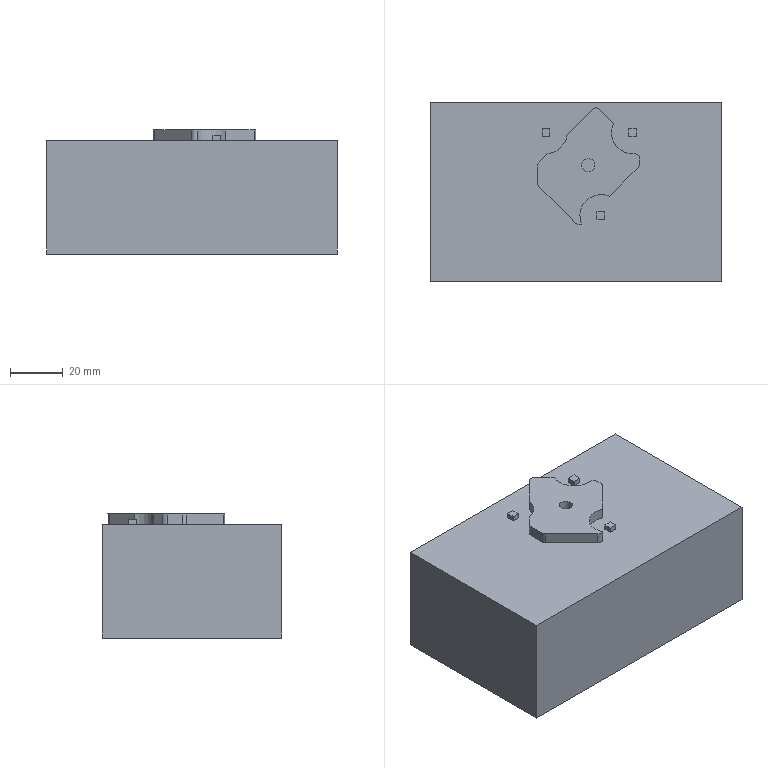NC program | NX | posted with a generic post | part box 110.151 x 68.163 x 47.1 mm
Lines 3425 to 4268 of 32691:
(PLANAR_MILL_2 , TOOL : D4R0)
N6680 T14 M6
N6682 G54
N6684 G17 G0 G90 X46.442 Y26.396 S5000 M3
N6686 G43 Z80. H14
N6688 G94 G1 Z0.5 F5000.
N6690 X46.014 Y26.643 Z0.487 F1500.
N6692 X45.498 Y26.638 Z0.474
N6694 X45.082 Y26.398 Z0.461
N6696 X44.819 Y25.953 Z0.447
N6698 Y25.437 Z0.434
N6700 X45.082 Y24.993 Z0.42
N6702 X45.498 Y24.752 Z0.408
N6704 X46.014 Y24.748 Z0.394
N6706 X46.461 Y25.005 Z0.381
N6708 X46.715 Y25.455 Z0.367
N6710 Y25.936 Z0.355
N6712 X46.461 Y26.385 Z0.341
N6714 X46.014 Y26.643 Z0.328
N6716 X45.498 Y26.638 Z0.314
N6718 X45.082 Y26.398 Z0.302
N6720 X44.819 Y25.953 Z0.288
N6722 Y25.437 Z0.275
N6724 X45.082 Y24.993 Z0.261
N6726 X45.498 Y24.752 Z0.248
N6728 X46.014 Y24.748 Z0.235
N6730 X46.461 Y25.005 Z0.221
N6732 X46.715 Y25.455 Z0.208
N6734 Y25.936 Z0.195
N6736 X46.461 Y26.385 Z0.182
N6738 X46.014 Y26.643 Z0.168
N6740 X45.498 Y26.638 Z0.155
N6742 X45.082 Y26.398 Z0.142
N6744 X44.819 Y25.953 Z0.129
N6746 Y25.437 Z0.115
N6748 X45.082 Y24.993 Z0.102
N6750 X45.498 Y24.752 Z0.089
N6752 X46.014 Y24.748 Z0.076
N6754 X46.461 Y25.005 Z0.062
N6756 X46.715 Y25.455 Z0.048
N6758 Y25.936 Z0.036
N6760 X46.461 Y26.385 Z0.022
N6762 X46.014 Y26.643 Z0.009
N6764 X45.498 Y26.638 Z-0.005
N6766 X45.082 Y26.398 Z-0.017
N6768 X44.819 Y25.953 Z-0.031
N6770 Y25.437 Z-0.044
N6772 X45.082 Y24.993 Z-0.058
N6774 X45.498 Y24.752 Z-0.07
N6776 X46.014 Y24.748 Z-0.084
N6778 X46.461 Y25.005 Z-0.097
N6780 X46.715 Y25.455 Z-0.111
N6782 Y25.936 Z-0.124
N6784 X46.461 Y26.385 Z-0.137
N6786 X46.014 Y26.643 Z-0.151
N6788 X45.498 Y26.638 Z-0.164
N6790 X45.082 Y26.398 Z-0.177
N6792 X44.819 Y25.953 Z-0.19
N6794 Y25.437 Z-0.204
N6796 X45.082 Y24.993 Z-0.217
N6798 X45.498 Y24.752 Z-0.23
N6800 X46.014 Y24.748 Z-0.243
N6802 X46.461 Y25.005 Z-0.257
N6804 X46.715 Y25.455 Z-0.27
N6806 Y25.936 Z-0.283
N6808 X46.461 Y26.385 Z-0.296
N6810 X46.014 Y26.643 Z-0.31
N6812 X45.498 Y26.638 Z-0.323
N6814 X45.082 Y26.398 Z-0.336
N6816 X44.819 Y25.953 Z-0.35
N6818 Y25.437 Z-0.363
N6820 X45.082 Y24.993 Z-0.377
N6822 X45.498 Y24.752 Z-0.389
N6824 X46.014 Y24.748 Z-0.403
N6826 X46.461 Y25.005 Z-0.416
N6828 X46.715 Y25.455 Z-0.43
N6830 Y25.936 Z-0.442
N6832 X46.461 Y26.385 Z-0.456
N6834 X46.014 Y26.643 Z-0.469
N6836 X45.498 Y26.638 Z-0.483
N6838 X45.082 Y26.398 Z-0.495
N6840 X44.819 Y25.953 Z-0.509
N6842 Y25.437 Z-0.522
N6844 X45.082 Y24.993 Z-0.536
N6846 X45.498 Y24.752 Z-0.549
N6848 X46.014 Y24.748 Z-0.562
N6850 X46.461 Y25.005 Z-0.576
N6852 X46.715 Y25.455 Z-0.589
N6854 Y25.936 Z-0.602
N6856 X46.461 Y26.385 Z-0.615
N6858 X46.014 Y26.643 Z-0.629
N6860 X45.498 Y26.638 Z-0.642
N6862 X45.082 Y26.398 Z-0.655
N6864 X44.819 Y25.953 Z-0.668
N6866 Y25.437 Z-0.682
N6868 X45.082 Y24.993 Z-0.695
N6870 X45.498 Y24.752 Z-0.708
N6872 X46.014 Y24.748 Z-0.721
N6874 X46.461 Y25.005 Z-0.735
N6876 X46.715 Y25.455 Z-0.749
N6878 Y25.936 Z-0.761
N6880 X46.461 Y26.385 Z-0.775
N6882 X46.014 Y26.643 Z-0.788
N6884 X45.498 Y26.638 Z-0.802
N6886 X45.082 Y26.398 Z-0.814
N6888 X44.819 Y25.953 Z-0.828
N6890 Y25.437 Z-0.841
N6892 X45.082 Y24.993 Z-0.855
N6894 X45.498 Y24.752 Z-0.867
N6896 X46.014 Y24.748 Z-0.881
N6898 X46.461 Y25.005 Z-0.894
N6900 X46.715 Y25.455 Z-0.908
N6902 Y25.936 Z-0.921
N6904 X46.461 Y26.385 Z-0.934
N6906 X46.014 Y26.643 Z-0.948
N6908 X45.498 Y26.638 Z-0.961
N6910 X45.082 Y26.398 Z-0.974
N6912 X44.819 Y25.953 Z-0.987
N6914 Y25.437 Z-1.001
N6916 X45.082 Y24.993 Z-1.014
N6918 X45.498 Y24.752 Z-1.027
N6920 X46.014 Y24.748 Z-1.04
N6922 X46.461 Y25.005 Z-1.054
N6924 X46.715 Y25.455 Z-1.067
N6926 Y25.936 Z-1.08
N6928 X46.461 Y26.385 Z-1.093
N6930 X46.014 Y26.643 Z-1.107
N6932 X45.498 Y26.638 Z-1.12
N6934 X45.082 Y26.398 Z-1.133
N6936 X44.819 Y25.953 Z-1.147
N6938 Y25.437 Z-1.16
N6940 X45.082 Y24.993 Z-1.174
N6942 X45.498 Y24.752 Z-1.186
N6944 X46.014 Y24.748 Z-1.2
N6946 X46.461 Y25.005 Z-1.213
N6948 X46.715 Y25.455 Z-1.227
N6950 Y25.936 Z-1.239
N6952 X46.461 Y26.385 Z-1.253
N6954 X46.014 Y26.643 Z-1.266
N6956 X45.498 Y26.638 Z-1.28
N6958 X45.082 Y26.398 Z-1.292
N6960 X44.819 Y25.953 Z-1.306
N6962 Y25.437 Z-1.319
N6964 X45.082 Y24.993 Z-1.333
N6966 X45.498 Y24.752 Z-1.346
N6968 X46.014 Y24.748 Z-1.359
N6970 X46.461 Y25.005 Z-1.373
N6972 X46.715 Y25.455 Z-1.386
N6974 Y25.936 Z-1.399
N6976 X46.461 Y26.385 Z-1.412
N6978 X46.014 Y26.643 Z-1.426
N6980 X45.498 Y26.638 Z-1.439
N6982 X45.082 Y26.398 Z-1.452
N6984 X44.819 Y25.953 Z-1.465
N6986 Y25.437 Z-1.479
N6988 X45.082 Y24.993 Z-1.492
N6990 X45.498 Y24.752 Z-1.505
N6992 X46.014 Y24.748 Z-1.518
N6994 X46.461 Y25.005 Z-1.532
N6996 X46.715 Y25.455 Z-1.546
N6998 Y25.936 Z-1.558
N7000 X46.461 Y26.385 Z-1.572
N7002 X46.014 Y26.643 Z-1.585
N7004 X45.498 Y26.638 Z-1.599
N7006 X45.082 Y26.398 Z-1.611
N7008 X44.819 Y25.953 Z-1.625
N7010 Y25.437 Z-1.638
N7012 X45.082 Y24.993 Z-1.652
N7014 X45.498 Y24.752 Z-1.664
N7016 X46.014 Y24.748 Z-1.678
N7018 X46.461 Y25.005 Z-1.691
N7020 X46.715 Y25.455 Z-1.705
N7022 Y25.936 Z-1.718
N7024 X46.461 Y26.385 Z-1.731
N7026 X46.014 Y26.643 Z-1.745
N7028 X45.498 Y26.638 Z-1.758
N7030 X45.082 Y26.398 Z-1.771
N7032 X44.819 Y25.953 Z-1.784
N7034 Y25.437 Z-1.798
N7036 X45.082 Y24.993 Z-1.811
N7038 X45.498 Y24.752 Z-1.824
N7040 X46.014 Y24.748 Z-1.837
N7042 X46.461 Y25.005 Z-1.851
N7044 X46.715 Y25.455 Z-1.864
N7046 Y25.936 Z-1.877
N7048 X46.461 Y26.385 Z-1.89
N7050 X46.014 Y26.643 Z-1.904
N7052 X45.498 Y26.638 Z-1.917
N7054 X45.082 Y26.398 Z-1.93
N7056 X44.819 Y25.953 Z-1.944
N7058 Y25.437 Z-1.957
N7060 X45.082 Y24.993 Z-1.971
N7062 X45.498 Y24.752 Z-1.983
N7064 X46.014 Y24.748 Z-1.997
N7066 X46.461 Y25.005 Z-2.01
N7068 X46.715 Y25.455 Z-2.024
N7070 Y25.936 Z-2.036
N7072 X46.461 Y26.385 Z-2.05
N7074 X46.014 Y26.643 Z-2.063
N7076 X45.498 Y26.638 Z-2.077
N7078 X45.082 Y26.398 Z-2.089
N7080 X44.819 Y25.953 Z-2.103
N7082 Y25.437 Z-2.116
N7084 X45.082 Y24.993 Z-2.13
N7086 X45.498 Y24.752 Z-2.143
N7088 X46.014 Y24.748 Z-2.156
N7090 X46.461 Y25.005 Z-2.17
N7092 X46.715 Y25.455 Z-2.183
N7094 Y25.936 Z-2.196
N7096 X46.461 Y26.385 Z-2.209
N7098 X46.014 Y26.643 Z-2.223
N7100 X45.498 Y26.638 Z-2.236
N7102 X45.082 Y26.398 Z-2.249
N7104 X44.819 Y25.953 Z-2.262
N7106 Y25.437 Z-2.276
N7108 X45.082 Y24.993 Z-2.289
N7110 X45.498 Y24.752 Z-2.302
N7112 X46.014 Y24.748 Z-2.315
N7114 X46.461 Y25.005 Z-2.329
N7116 X46.715 Y25.455 Z-2.343
N7118 Y25.936 Z-2.355
N7120 X46.461 Y26.385 Z-2.369
N7122 X46.014 Y26.643 Z-2.382
N7124 X45.498 Y26.638 Z-2.396
N7126 X45.082 Y26.398 Z-2.408
N7128 X44.819 Y25.953 Z-2.422
N7130 Y25.437 Z-2.435
N7132 X45.082 Y24.993 Z-2.449
N7134 X45.498 Y24.752 Z-2.461
N7136 X46.014 Y24.748 Z-2.475
N7138 X46.461 Y25.005 Z-2.488
N7140 X46.715 Y25.455 Z-2.502
N7142 Y25.936 Z-2.515
N7144 X46.461 Y26.385 Z-2.528
N7146 X46.014 Y26.643 Z-2.542
N7148 X45.498 Y26.638 Z-2.555
N7150 X45.082 Y26.398 Z-2.568
N7152 X44.819 Y25.953 Z-2.581
N7154 Y25.437 Z-2.595
N7156 X45.082 Y24.993 Z-2.608
N7158 X45.498 Y24.752 Z-2.621
N7160 X46.014 Y24.748 Z-2.634
N7162 X46.461 Y25.005 Z-2.648
N7164 X46.715 Y25.455 Z-2.661
N7166 Y25.936 Z-2.674
N7168 X46.461 Y26.385 Z-2.687
N7170 X46.014 Y26.643 Z-2.701
N7172 X45.498 Y26.638 Z-2.714
N7174 X45.082 Y26.398 Z-2.727
N7176 X44.819 Y25.953 Z-2.741
N7178 Y25.437 Z-2.754
N7180 X45.082 Y24.993 Z-2.768
N7182 X45.498 Y24.752 Z-2.78
N7184 X46.014 Y24.748 Z-2.794
N7186 X46.461 Y25.005 Z-2.807
N7188 X46.715 Y25.455 Z-2.821
N7190 Y25.936 Z-2.833
N7192 X46.461 Y26.385 Z-2.847
N7194 X46.014 Y26.643 Z-2.86
N7196 X45.498 Y26.638 Z-2.874
N7198 X45.082 Y26.398 Z-2.886
N7200 X44.819 Y25.953 Z-2.9
N7202 Y25.437 Z-2.913
N7204 X45.082 Y24.993 Z-2.927
N7206 X45.498 Y24.752 Z-2.94
N7208 X46.014 Y24.748 Z-2.953
N7210 X46.461 Y25.005 Z-2.967
N7212 X46.715 Y25.455 Z-2.98
N7214 Y25.936 Z-2.993
N7216 X46.461 Y26.385 Z-3.006
N7218 X46.014 Y26.643 Z-3.02
N7220 X45.498 Y26.638 Z-3.033
N7222 X45.082 Y26.398 Z-3.046
N7224 X44.819 Y25.953 Z-3.059
N7226 Y25.437 Z-3.073
N7228 X45.082 Y24.993 Z-3.086
N7230 X45.498 Y24.752 Z-3.099
N7232 X46.014 Y24.748 Z-3.112
N7234 X46.461 Y25.005 Z-3.126
N7236 X46.715 Y25.455 Z-3.14
N7238 Y25.936 Z-3.152
N7240 X46.461 Y26.385 Z-3.166
N7242 X46.014 Y26.643 Z-3.179
N7244 X45.498 Y26.638 Z-3.193
N7246 X45.082 Y26.398 Z-3.205
N7248 X44.819 Y25.953 Z-3.219
N7250 Y25.437 Z-3.232
N7252 X45.082 Y24.993 Z-3.246
N7254 X45.498 Y24.752 Z-3.258
N7256 X46.014 Y24.748 Z-3.272
N7258 X46.461 Y25.005 Z-3.285
N7260 X46.715 Y25.455 Z-3.299
N7262 Y25.936 Z-3.312
N7264 X46.461 Y26.385 Z-3.325
N7266 X46.014 Y26.643 Z-3.339
N7268 X45.498 Y26.638 Z-3.352
N7270 X45.082 Y26.398 Z-3.365
N7272 X44.819 Y25.953 Z-3.378
N7274 Y25.437 Z-3.392
N7276 X45.082 Y24.993 Z-3.405
N7278 X45.498 Y24.752 Z-3.418
N7280 X46.014 Y24.748 Z-3.431
N7282 X46.461 Y25.005 Z-3.445
N7284 X46.715 Y25.455 Z-3.458
N7286 Y25.936 Z-3.471
N7288 X46.461 Y26.385 Z-3.484
N7290 X46.014 Y26.643 Z-3.498
N7292 X45.498 Y26.638 Z-3.511
N7294 X45.082 Y26.398 Z-3.524
N7296 X44.819 Y25.953 Z-3.538
N7298 Y25.437 Z-3.551
N7300 X45.082 Y24.993 Z-3.565
N7302 X45.498 Y24.752 Z-3.577
N7304 X46.014 Y24.748 Z-3.591
N7306 X46.461 Y25.005 Z-3.604
N7308 X46.715 Y25.455 Z-3.618
N7310 Y25.936 Z-3.63
N7312 X46.461 Y26.385 Z-3.644
N7314 X46.014 Y26.643 Z-3.657
N7316 X45.498 Y26.638 Z-3.671
N7318 X45.082 Y26.398 Z-3.683
N7320 X44.819 Y25.953 Z-3.697
N7322 Y25.437 Z-3.71
N7324 X45.082 Y24.993 Z-3.724
N7326 X45.498 Y24.752 Z-3.737
N7328 X46.014 Y24.748 Z-3.75
N7330 X46.461 Y25.005 Z-3.764
N7332 X46.715 Y25.455 Z-3.777
N7334 Y25.936 Z-3.79
N7336 X46.461 Y26.385 Z-3.803
N7338 X46.014 Y26.643 Z-3.817
N7340 X45.498 Y26.638 Z-3.83
N7342 X45.082 Y26.398 Z-3.843
N7344 X44.819 Y25.953 Z-3.856
N7346 Y25.437 Z-3.87
N7348 X45.082 Y24.993 Z-3.883
N7350 X45.498 Y24.752 Z-3.896
N7352 X46.014 Y24.748 Z-3.909
N7354 X46.461 Y25.005 Z-3.923
N7356 X46.715 Y25.455 Z-3.937
N7358 Y25.936 Z-3.949
N7360 X46.461 Y26.385 Z-3.963
N7362 X46.014 Y26.643 Z-3.976
N7364 X45.498 Y26.638 Z-3.99
N7366 X45.082 Y26.398 Z-4.002
N7368 X44.819 Y25.953 Z-4.016
N7370 Y25.437 Z-4.029
N7372 X45.082 Y24.993 Z-4.043
N7374 X45.498 Y24.752 Z-4.055
N7376 X46.014 Y24.748 Z-4.069
N7378 X46.461 Y25.005 Z-4.082
N7380 X46.715 Y25.455 Z-4.096
N7382 Y25.936 Z-4.109
N7384 X46.461 Y26.385 Z-4.122
N7386 X46.014 Y26.643 Z-4.136
N7388 X45.498 Y26.638 Z-4.149
N7390 X45.082 Y26.398 Z-4.162
N7392 X44.819 Y25.953 Z-4.175
N7394 Y25.437 Z-4.189
N7396 X45.082 Y24.993 Z-4.202
N7398 X45.498 Y24.752 Z-4.215
N7400 X46.014 Y24.748 Z-4.228
N7402 X46.461 Y25.005 Z-4.242
N7404 X46.715 Y25.455 Z-4.255
N7406 Y25.936 Z-4.268
N7408 X46.461 Y26.385 Z-4.281
N7410 X46.014 Y26.643 Z-4.295
N7412 X45.498 Y26.638 Z-4.308
N7414 X45.082 Y26.398 Z-4.321
N7416 X44.819 Y25.953 Z-4.335
N7418 Y25.437 Z-4.348
N7420 X45.082 Y24.993 Z-4.362
N7422 X45.498 Y24.752 Z-4.374
N7424 X46.014 Y24.748 Z-4.388
N7426 X46.461 Y25.005 Z-4.401
N7428 X46.715 Y25.455 Z-4.415
N7430 Y25.936 Z-4.427
N7432 X46.461 Y26.385 Z-4.441
N7434 X46.014 Y26.643 Z-4.454
N7436 X45.498 Y26.638 Z-4.468
N7438 X45.082 Y26.398 Z-4.48
N7440 X44.819 Y25.953 Z-4.494
N7442 Y25.437 Z-4.507
N7444 X45.082 Y24.993 Z-4.521
N7446 X45.498 Y24.752 Z-4.534
N7448 X46.014 Y24.748 Z-4.547
N7450 X46.461 Y25.005 Z-4.561
N7452 X46.715 Y25.455 Z-4.574
N7454 Y25.936 Z-4.587
N7456 X46.461 Y26.385 Z-4.6
N7458 X46.014 Y26.643 Z-4.614
N7460 X45.498 Y26.638 Z-4.627
N7462 X45.082 Y26.398 Z-4.64
N7464 X44.819 Y25.953 Z-4.653
N7466 Y25.437 Z-4.667
N7468 X45.082 Y24.993 Z-4.68
N7470 X45.498 Y24.752 Z-4.693
N7472 X46.014 Y24.748 Z-4.706
N7474 X46.461 Y25.005 Z-4.72
N7476 X46.715 Y25.455 Z-4.734
N7478 Y25.936 Z-4.746
N7480 X46.461 Y26.385 Z-4.76
N7482 X46.014 Y26.643 Z-4.773
N7484 X45.498 Y26.638 Z-4.787
N7486 X45.082 Y26.398 Z-4.799
N7488 X44.819 Y25.953 Z-4.813
N7490 Y25.437 Z-4.826
N7492 X45.082 Y24.993 Z-4.84
N7494 X45.498 Y24.752 Z-4.852
N7496 X46.014 Y24.748 Z-4.866
N7498 X46.461 Y25.005 Z-4.879
N7500 X46.715 Y25.455 Z-4.893
N7502 Y25.936 Z-4.906
N7504 X46.461 Y26.385 Z-4.919
N7506 X46.014 Y26.643 Z-4.933
N7508 X45.498 Y26.638 Z-4.946
N7510 X45.082 Y26.398 Z-4.959
N7512 X44.819 Y25.953 Z-4.972
N7514 Y25.437 Z-4.986
N7516 X45.082 Y24.993 Z-4.999
N7518 X45.498 Y24.752 Z-5.012
N7520 X46.014 Y24.748 Z-5.025
N7522 X46.461 Y25.005 Z-5.039
N7524 X46.715 Y25.455 Z-5.052
N7526 Y25.936 Z-5.065
N7528 X46.461 Y26.385 Z-5.078
N7530 X46.014 Y26.643 Z-5.092
N7532 X45.498 Y26.638 Z-5.105
N7534 X45.082 Y26.398 Z-5.118
N7536 X44.819 Y25.953 Z-5.132
N7538 Y25.437 Z-5.145
N7540 X45.082 Y24.993 Z-5.159
N7542 X45.498 Y24.752 Z-5.171
N7544 X46.014 Y24.748 Z-5.185
N7546 X46.461 Y25.005 Z-5.198
N7548 X46.715 Y25.455 Z-5.212
N7550 Y25.936 Z-5.224
N7552 X46.461 Y26.385 Z-5.238
N7554 X46.014 Y26.643 Z-5.251
N7556 X45.498 Y26.638 Z-5.265
N7558 X45.082 Y26.398 Z-5.277
N7560 X44.819 Y25.953 Z-5.291
N7562 Y25.437 Z-5.304
N7564 X45.082 Y24.993 Z-5.318
N7566 X45.498 Y24.752 Z-5.331
N7568 X46.014 Y24.748 Z-5.344
N7570 X46.461 Y25.005 Z-5.358
N7572 X46.715 Y25.455 Z-5.371
N7574 Y25.936 Z-5.384
N7576 X46.461 Y26.385 Z-5.397
N7578 X46.014 Y26.643 Z-5.411
N7580 X45.498 Y26.638 Z-5.424
N7582 X45.082 Y26.398 Z-5.437
N7584 X44.819 Y25.953 Z-5.45
N7586 Y25.437 Z-5.464
N7588 X45.082 Y24.993 Z-5.477
N7590 X45.498 Y24.752 Z-5.49
N7592 X46.014 Y24.748 Z-5.503
N7594 X46.461 Y25.005 Z-5.517
N7596 X46.715 Y25.455 Z-5.531
N7598 Y25.936 Z-5.543
N7600 X46.461 Y26.385 Z-5.557
N7602 X46.014 Y26.643 Z-5.57
N7604 X45.498 Y26.638 Z-5.584
N7606 X45.082 Y26.398 Z-5.596
N7608 X44.819 Y25.953 Z-5.61
N7610 Y25.437 Z-5.623
N7612 X45.082 Y24.993 Z-5.637
N7614 X45.498 Y24.752 Z-5.649
N7616 X46.014 Y24.748 Z-5.663
N7618 X46.461 Y25.005 Z-5.676
N7620 X46.715 Y25.455 Z-5.69
N7622 Y25.936 Z-5.703
N7624 X46.461 Y26.385 Z-5.716
N7626 X46.014 Y26.643 Z-5.73
N7628 X45.498 Y26.638 Z-5.743
N7630 X45.082 Y26.398 Z-5.756
N7632 X44.819 Y25.953 Z-5.769
N7634 Y25.437 Z-5.783
N7636 X45.082 Y24.993 Z-5.796
N7638 X45.498 Y24.752 Z-5.809
N7640 X46.014 Y24.748 Z-5.822
N7642 X46.461 Y25.005 Z-5.836
N7644 X46.715 Y25.455 Z-5.849
N7646 Y25.936 Z-5.862
N7648 X46.461 Y26.385 Z-5.875
N7650 X46.014 Y26.643 Z-5.889
N7652 X45.498 Y26.638 Z-5.902
N7654 X45.082 Y26.398 Z-5.915
N7656 X44.819 Y25.953 Z-5.929
N7658 Y25.437 Z-5.942
N7660 X45.082 Y24.993 Z-5.956
N7662 X45.498 Y24.752 Z-5.968
N7664 X46.014 Y24.748 Z-5.982
N7666 X46.461 Y25.005 Z-5.995
N7668 X46.715 Y25.455 Z-6.009
N7670 Y25.936 Z-6.021
N7672 X46.461 Y26.385 Z-6.035
N7674 X46.014 Y26.643 Z-6.048
N7676 X45.498 Y26.638 Z-6.062
N7678 X45.082 Y26.398 Z-6.074
N7680 X44.819 Y25.953 Z-6.088
N7682 Y25.437 Z-6.101
N7684 X45.082 Y24.993 Z-6.115
N7686 X45.498 Y24.752 Z-6.128
N7688 X46.014 Y24.748 Z-6.141
N7690 X46.461 Y25.005 Z-6.155
N7692 X46.715 Y25.455 Z-6.168
N7694 Y25.936 Z-6.181
N7696 X46.461 Y26.385 Z-6.194
N7698 X46.014 Y26.643 Z-6.208
N7700 X45.498 Y26.638 Z-6.221
N7702 X45.082 Y26.398 Z-6.234
N7704 X44.819 Y25.953 Z-6.247
N7706 Y25.437 Z-6.261
N7708 X45.082 Y24.993 Z-6.274
N7710 X45.498 Y24.752 Z-6.287
N7712 X46.014 Y24.748 Z-6.3
N7714 X46.461 Y25.005 Z-6.314
N7716 X46.715 Y25.455 Z-6.328
N7718 Y25.936 Z-6.34
N7720 X46.461 Y26.385 Z-6.354
N7722 X46.014 Y26.643 Z-6.367
N7724 X45.498 Y26.638 Z-6.381
N7726 X45.082 Y26.398 Z-6.393
N7728 X44.819 Y25.953 Z-6.407
N7730 Y25.437 Z-6.42
N7732 X45.082 Y24.993 Z-6.434
N7734 X45.498 Y24.752 Z-6.446
N7736 X46.014 Y24.748 Z-6.46
N7738 X46.461 Y25.005 Z-6.473
N7740 X46.715 Y25.455 Z-6.487
N7742 Y25.936 Z-6.5
N7744 X46.461 Y26.385 Z-6.513
N7746 X46.014 Y26.643 Z-6.527
N7748 X45.498 Y26.638 Z-6.54
N7750 X45.082 Y26.398 Z-6.553
N7752 X44.819 Y25.953 Z-6.566
N7754 Y25.437 Z-6.58
N7756 X45.082 Y24.993 Z-6.593
N7758 X45.498 Y24.752 Z-6.606
N7760 X46.014 Y24.748 Z-6.619
N7762 X46.461 Y25.005 Z-6.633
N7764 X46.715 Y25.455 Z-6.646
N7766 Y25.936 Z-6.659
N7768 X46.461 Y26.385 Z-6.672
N7770 X46.014 Y26.643 Z-6.686
N7772 X45.498 Y26.638 Z-6.699
N7774 X45.082 Y26.398 Z-6.712
N7776 X44.819 Y25.953 Z-6.726
N7778 Y25.437 Z-6.739
N7780 X45.082 Y24.993 Z-6.753
N7782 X45.498 Y24.752 Z-6.765
N7784 X46.014 Y24.748 Z-6.779
N7786 X46.461 Y25.005 Z-6.792
N7788 X46.715 Y25.455 Z-6.806
N7790 Y25.936 Z-6.818
N7792 X46.461 Y26.385 Z-6.832
N7794 X46.014 Y26.643 Z-6.845
N7796 X45.498 Y26.638 Z-6.859
N7798 X45.082 Y26.398 Z-6.871
N7800 X44.819 Y25.953 Z-6.885
N7802 Y25.437 Z-6.898
N7804 X45.082 Y24.993 Z-6.912
N7806 X45.498 Y24.752 Z-6.925
N7808 X46.014 Y24.748 Z-6.938
N7810 X46.461 Y25.005 Z-6.952
N7812 X46.715 Y25.455 Z-6.965
N7814 Y25.936 Z-6.978
N7816 X46.461 Y26.385 Z-6.991
N7818 X46.014 Y26.643 Z-7.005
N7820 X45.498 Y26.638 Z-7.018
N7822 X45.082 Y26.398 Z-7.031
N7824 X44.819 Y25.953 Z-7.044
N7826 Y25.437 Z-7.058
N7828 X45.082 Y24.993 Z-7.071
N7830 X45.498 Y24.752 Z-7.084
N7832 X46.014 Y24.748 Z-7.097
N7834 X46.461 Y25.005 Z-7.111
N7836 X46.715 Y25.455 Z-7.125
N7838 Y25.936 Z-7.137
N7840 X46.461 Y26.385 Z-7.151
N7842 X46.014 Y26.643 Z-7.164
N7844 X45.498 Y26.638 Z-7.178
N7846 X45.082 Y26.398 Z-7.19
N7848 X44.819 Y25.953 Z-7.204
N7850 Y25.437 Z-7.217
N7852 X45.082 Y24.993 Z-7.231
N7854 X45.498 Y24.752 Z-7.243
N7856 X46.014 Y24.748 Z-7.257
N7858 X46.461 Y25.005 Z-7.27
N7860 X46.715 Y25.455 Z-7.284
N7862 Y25.936 Z-7.297
N7864 X46.461 Y26.385 Z-7.31
N7866 X46.014 Y26.643 Z-7.324
N7868 X45.498 Y26.638 Z-7.337
N7870 X45.082 Y26.398 Z-7.35
N7872 X44.819 Y25.953 Z-7.363
N7874 Y25.437 Z-7.377
N7876 X45.082 Y24.993 Z-7.39
N7878 X45.498 Y24.752 Z-7.403
N7880 X46.014 Y24.748 Z-7.416
N7882 X46.461 Y25.005 Z-7.43
N7884 X46.715 Y25.455 Z-7.443
N7886 Y25.936 Z-7.456
N7888 X46.461 Y26.385 Z-7.469
N7890 X46.014 Y26.643 Z-7.483
N7892 X45.498 Y26.638 Z-7.496
N7894 X45.082 Y26.398 Z-7.509
N7896 X44.819 Y25.953 Z-7.523
N7898 Y25.437 Z-7.536
N7900 X45.082 Y24.993 Z-7.55
N7902 X45.498 Y24.752 Z-7.562
N7904 X46.014 Y24.748 Z-7.576
N7906 X46.461 Y25.005 Z-7.589
N7908 X46.715 Y25.455 Z-7.603
N7910 Y25.936 Z-7.615
N7912 X46.461 Y26.385 Z-7.629
N7914 X46.014 Y26.643 Z-7.642
N7916 X45.498 Y26.638 Z-7.656
N7918 X45.082 Y26.398 Z-7.668
N7920 X44.819 Y25.953 Z-7.682
N7922 Y25.437 Z-7.695
N7924 X45.082 Y24.993 Z-7.709
N7926 X45.498 Y24.752 Z-7.722
N7928 X46.014 Y24.748 Z-7.735
N7930 X46.461 Y25.005 Z-7.749
N7932 X46.715 Y25.455 Z-7.762
N7934 Y25.936 Z-7.775
N7936 X46.461 Y26.385 Z-7.788
N7938 X46.014 Y26.643 Z-7.802
N7940 X45.498 Y26.638 Z-7.815
N7942 X45.082 Y26.398 Z-7.828
N7944 X44.819 Y25.953 Z-7.841
N7946 Y25.437 Z-7.855
N7948 X45.082 Y24.993 Z-7.868
N7950 X45.498 Y24.752 Z-7.881
N7952 X46.014 Y24.748 Z-7.894
N7954 X46.461 Y25.005 Z-7.908
N7956 X46.715 Y25.455 Z-7.922
N7958 Y25.936 Z-7.934
N7960 X46.461 Y26.385 Z-7.948
N7962 X46.014 Y26.643 Z-7.961
N7964 X45.498 Y26.638 Z-7.975
N7966 X45.082 Y26.398 Z-7.987
N7968 X44.819 Y25.953 Z-8.001
N7970 Y25.437 Z-8.014
N7972 X45.082 Y24.993 Z-8.028
N7974 X45.498 Y24.752 Z-8.04
N7976 X46.014 Y24.748 Z-8.054
N7978 X46.461 Y25.005 Z-8.067
N7980 X46.715 Y25.455 Z-8.081
N7982 Y25.936 Z-8.094
N7984 X46.461 Y26.385 Z-8.107
N7986 X46.014 Y26.643 Z-8.121
N7988 X45.498 Y26.638 Z-8.134
N7990 X45.082 Y26.398 Z-8.147
N7992 X44.819 Y25.953 Z-8.16
N7994 Y25.437 Z-8.174
N7996 X45.082 Y24.993 Z-8.187
N7998 X45.498 Y24.752 Z-8.2
N8000 X46.014 Y24.748 Z-8.213
N8002 X46.461 Y25.005 Z-8.227
N8004 X46.715 Y25.455 Z-8.24
N8006 Y25.936 Z-8.253
N8008 X46.461 Y26.385 Z-8.266
N8010 X46.014 Y26.643 Z-8.28
N8012 X45.498 Y26.638 Z-8.293
N8014 X45.082 Y26.398 Z-8.306
N8016 X44.819 Y25.953 Z-8.32
N8018 Y25.437 Z-8.333
N8020 X45.082 Y24.993 Z-8.347
N8022 X45.498 Y24.752 Z-8.359
N8024 X46.014 Y24.748 Z-8.373
N8026 X46.461 Y25.005 Z-8.386
N8028 X46.715 Y25.455 Z-8.4
N8030 Y25.936 Z-8.412
N8032 X46.461 Y26.385 Z-8.426
N8034 X46.014 Y26.643 Z-8.439
N8036 X45.498 Y26.638 Z-8.453
N8038 X45.082 Y26.398 Z-8.465
N8040 X44.819 Y25.953 Z-8.479
N8042 Y25.437 Z-8.492
N8044 X45.082 Y24.993 Z-8.506
N8046 X45.498 Y24.752 Z-8.519
N8048 X46.014 Y24.748 Z-8.532
N8050 X46.461 Y25.005 Z-8.546
N8052 X46.715 Y25.455 Z-8.559
N8054 Y25.936 Z-8.572
N8056 X46.461 Y26.385 Z-8.585
N8058 X46.014 Y26.643 Z-8.599
N8060 X45.498 Y26.638 Z-8.612
N8062 X45.082 Y26.398 Z-8.625
N8064 X44.819 Y25.953 Z-8.638
N8066 Y25.437 Z-8.652
N8068 X45.082 Y24.993 Z-8.665
N8070 X45.498 Y24.752 Z-8.678
N8072 X46.014 Y24.748 Z-8.691
N8074 X46.461 Y25.005 Z-8.705
N8076 X46.715 Y25.455 Z-8.719
N8078 Y25.936 Z-8.731
N8080 X46.461 Y26.385 Z-8.745
N8082 X46.014 Y26.643 Z-8.758
N8084 X45.498 Y26.638 Z-8.772
N8086 X45.082 Y26.398 Z-8.784
N8088 X44.819 Y25.953 Z-8.798
N8090 Y25.437 Z-8.811
N8092 X45.082 Y24.993 Z-8.825
N8094 X45.498 Y24.752 Z-8.837
N8096 X46.014 Y24.748 Z-8.851
N8098 X46.461 Y25.005 Z-8.864
N8100 X46.715 Y25.455 Z-8.878
N8102 Y25.936 Z-8.891
N8104 X46.461 Y26.385 Z-8.904
N8106 X46.014 Y26.643 Z-8.918
N8108 X45.498 Y26.638 Z-8.931
N8110 X45.082 Y26.398 Z-8.944
N8112 X44.819 Y25.953 Z-8.957
N8114 Y25.437 Z-8.971
N8116 X45.082 Y24.993 Z-8.984
N8118 X45.498 Y24.752 Z-8.997
N8120 X46.014 Y24.748 Z-9.01
N8122 X46.461 Y25.005 Z-9.024
N8124 X46.715 Y25.455 Z-9.037
N8126 Y25.936 Z-9.05
N8128 X46.461 Y26.385 Z-9.063
N8130 X46.014 Y26.643 Z-9.077
N8132 X45.498 Y26.638 Z-9.09
N8134 X45.082 Y26.398 Z-9.103
N8136 X44.819 Y25.953 Z-9.117
N8138 Y25.437 Z-9.13
N8140 X45.082 Y24.993 Z-9.144
N8142 X45.498 Y24.752 Z-9.156
N8144 X46.014 Y24.748 Z-9.17
N8146 X46.461 Y25.005 Z-9.183
N8148 X46.715 Y25.455 Z-9.197
N8150 Y25.936 Z-9.209
N8152 X46.461 Y26.385 Z-9.223
N8154 X46.014 Y26.643 Z-9.236
N8156 X45.498 Y26.638 Z-9.25
N8158 X45.082 Y26.398 Z-9.262
N8160 X44.819 Y25.953 Z-9.276
N8162 Y25.437 Z-9.289
N8164 X45.082 Y24.993 Z-9.303
N8166 X45.498 Y24.752 Z-9.316
N8168 X46.014 Y24.748 Z-9.329
N8170 X46.461 Y25.005 Z-9.343
N8172 X46.715 Y25.455 Z-9.356
N8174 Y25.936 Z-9.369
N8176 X46.461 Y26.385 Z-9.382
N8178 X46.014 Y26.643 Z-9.396
N8180 X45.498 Y26.638 Z-9.409
N8182 X45.082 Y26.398 Z-9.422
N8184 X44.819 Y25.953 Z-9.435
N8186 Y25.437 Z-9.449
N8188 X45.082 Y24.993 Z-9.462
N8190 X45.498 Y24.752 Z-9.475
N8192 X46.014 Y24.748 Z-9.488
N8194 X46.461 Y25.005 Z-9.502
N8196 X46.715 Y25.455 Z-9.516
N8198 Y25.936 Z-9.528
N8200 X46.461 Y26.385 Z-9.542
N8202 X46.014 Y26.643 Z-9.555
N8204 X45.498 Y26.638 Z-9.569
N8206 X45.082 Y26.398 Z-9.581
N8208 X44.819 Y25.953 Z-9.595
N8210 Y25.437 Z-9.608
N8212 X45.082 Y24.993 Z-9.622
N8214 X45.498 Y24.752 Z-9.634
N8216 X46.014 Y24.748 Z-9.648
N8218 X46.461 Y25.005 Z-9.661
N8220 X46.715 Y25.455 Z-9.675
N8222 Y25.936 Z-9.688
N8224 X46.461 Y26.385 Z-9.701
N8226 X46.014 Y26.643 Z-9.715
N8228 X45.498 Y26.638 Z-9.728
N8230 X45.082 Y26.398 Z-9.741
N8232 X44.819 Y25.953 Z-9.754
N8234 Y25.437 Z-9.768
N8236 X45.082 Y24.993 Z-9.781
N8238 X45.498 Y24.752 Z-9.794
N8240 X46.014 Y24.748 Z-9.807
N8242 X46.461 Y25.005 Z-9.821
N8244 X46.715 Y25.455 Z-9.834
N8246 Y25.936 Z-9.847
N8248 X46.461 Y26.385 Z-9.86
N8250 X46.014 Y26.643 Z-9.874
N8252 X45.498 Y26.638 Z-9.887
N8254 X45.082 Y26.398 Z-9.9
N8256 X44.819 Y25.953 Z-9.914
N8258 Y25.437 Z-9.927
N8260 X45.082 Y24.993 Z-9.941
N8262 X45.498 Y24.752 Z-9.953
N8264 X46.014 Y24.748 Z-9.967
N8266 X46.461 Y25.005 Z-9.98
N8268 X46.715 Y25.455 Z-9.994
N8270 Y25.695 Z-10.
N8272 G3 X45.765 Y26.645 R0.95
N8274 X46.715 Y25.695 R-0.95
N8276 G1 X46.315
N8278 G0 Z80.
N8280 X-36.937 Y-25.958
N8282 G1 Z0.5 F5000.
N8284 X-36.519 Y-26.201 Z0.487 F1500.
N8286 X-36.003 Y-26.206 Z0.474
N8288 X-35.556 Y-25.948 Z0.46
N8290 X-35.302 Y-25.499 Z0.447
N8292 Y-25.018 Z0.434
N8294 X-35.556 Y-24.568 Z0.421
N8296 X-36.003 Y-24.31 Z0.407
N8298 X-36.519 Y-24.315 Z0.394
N8300 X-36.936 Y-24.556 Z0.381
N8302 X-37.202 Y-25.018 Z0.367
N8304 Y-25.499 Z0.354
N8306 X-36.936 Y-25.961 Z0.341
N8308 X-36.519 Y-26.201 Z0.328
N8310 X-36.003 Y-26.206 Z0.314
N8312 X-35.556 Y-25.948 Z0.301
N8314 X-35.302 Y-25.499 Z0.287
N8316 Y-25.018 Z0.275
N8318 X-35.556 Y-24.568 Z0.261
N8320 X-36.003 Y-24.31 Z0.248
N8322 X-36.519 Y-24.315 Z0.234
N8324 X-36.936 Y-24.556 Z0.222
N8326 X-37.202 Y-25.018 Z0.208
N8328 Y-25.499 Z0.195
N8330 X-36.936 Y-25.961 Z0.181
N8332 X-36.519 Y-26.201 Z0.169
N8334 X-36.003 Y-26.206 Z0.155
N8336 X-35.556 Y-25.948 Z0.141
N8338 X-35.302 Y-25.499 Z0.128
N8340 Y-25.018 Z0.115
N8342 X-35.556 Y-24.568 Z0.102
N8344 X-36.003 Y-24.31 Z0.088
N8346 X-36.519 Y-24.315 Z0.075
N8348 X-36.936 Y-24.556 Z0.062
N8350 X-37.202 Y-25.018 Z0.048
N8352 Y-25.499 Z0.036
N8354 X-36.936 Y-25.961 Z0.022
N8356 X-36.519 Y-26.201 Z0.009
N8358 X-36.003 Y-26.206 Z-0.004
N8360 X-35.556 Y-25.948 Z-0.018